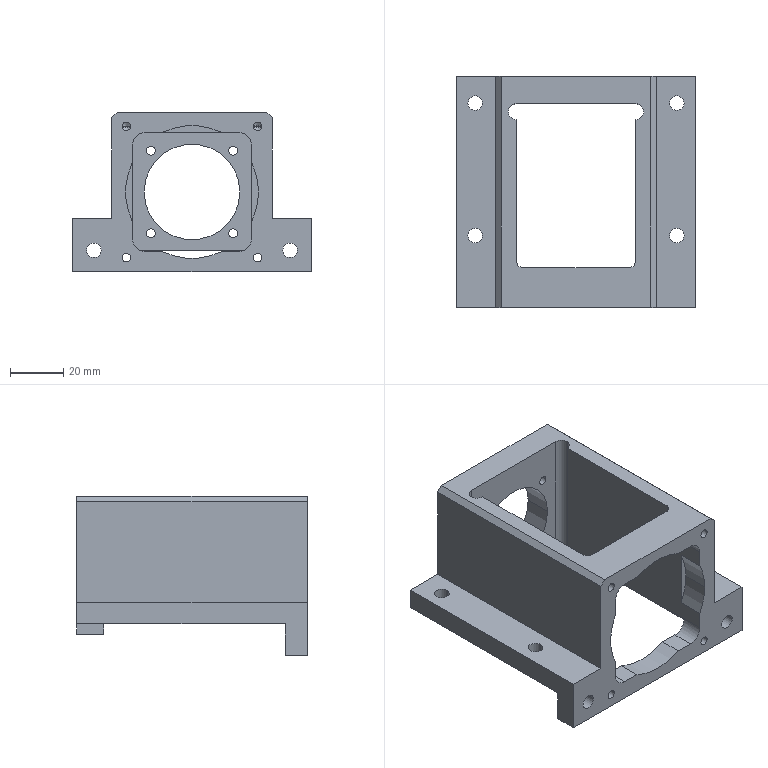Part | 1 solid | 78 faces | box 90 x 87.1 x 60 mm | volume 106559 mm3 | cylinder 44 | plane 30 | cone 4 | commonest cylinder face diameters 3.3 x16 5.5 x12 50.1 x5 10 x4 6 x3 5 x2